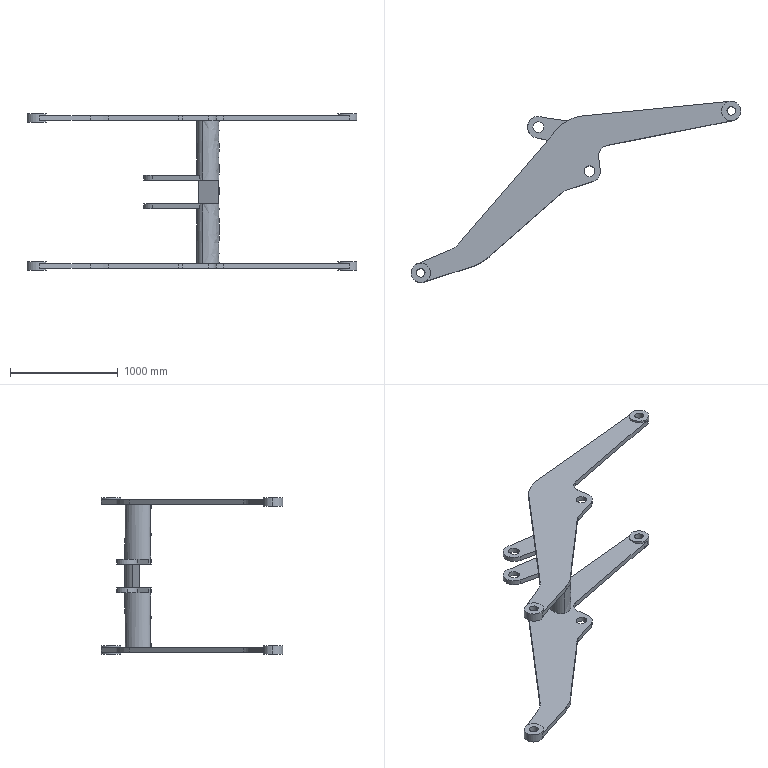Part | SolidWorks | features ICE 8, MirrorPattern 2, Cut 1, Extrusion 1 | 1 solid | 79 faces | box 3058 x 1680 x 1452 mm | volume 154389748 mm3 | cylinder 41 | plane 36 | spline 2 | commonest cylinder face diameters 200 x11 80 x8 100 x8 180 x8 700 x4 400 x2